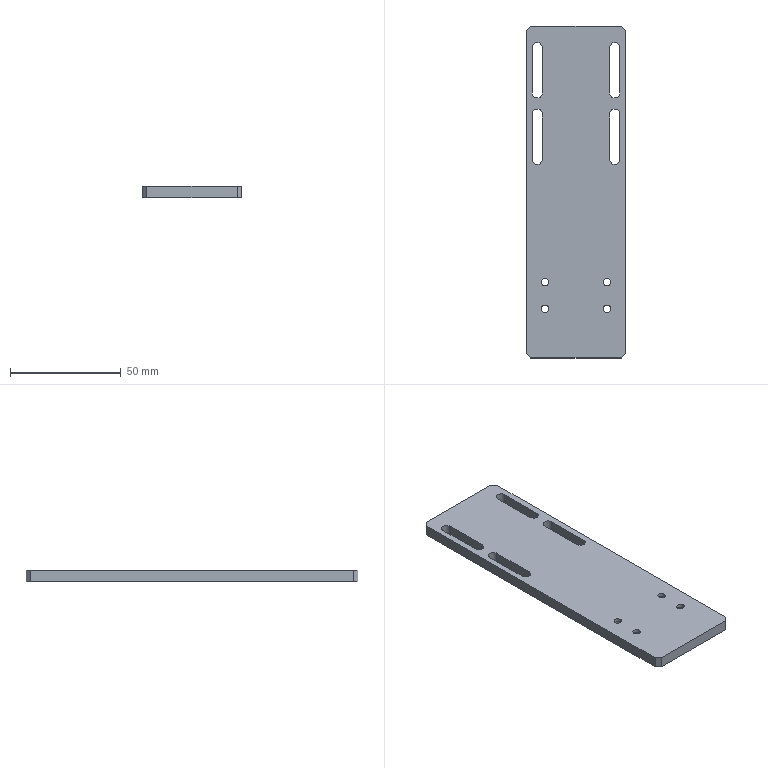Part | SolidWorks | features BaseBody 1 | 1 solid | 46 faces | box 45 x 150 x 5 mm | volume 31104 mm3 | cylinder 24 | plane 22 | commonest cylinder face diameters 3.4 x8 4.5 x8 6 x8
STEP:
#1=CARTESIAN_POINT('',(17.,-40.75,3.4));
#2=VERTEX_POINT('',#1);
#3=CARTESIAN_POINT('',(11.,-40.75,3.4));
#4=VERTEX_POINT('',#3);
#5=CARTESIAN_POINT('',(14.,-40.75,3.4));
#6=DIRECTION('',(0.,0.,-1.));
#7=DIRECTION('',(-1.,0.,0.));
#8=AXIS2_PLACEMENT_3D('',#5,#6,#7);
#9=CIRCLE('',#8,3.);
#10=EDGE_CURVE('',#2,#4,#9,.T.);
#11=ORIENTED_EDGE('',*,*,#10,.F.);
#12=CARTESIAN_POINT('',(17.,-40.75,0.));
#13=VERTEX_POINT('',#12);
#14=CARTESIAN_POINT('',(17.,-40.75,0.));
#15=DIRECTION('',(0.,0.,-1.));
#16=VECTOR('',#15,1000.);
#17=LINE('',#14,#16);
#18=EDGE_CURVE('',#2,#13,#17,.T.);
#19=ORIENTED_EDGE('',*,*,#18,.T.);
#20=CARTESIAN_POINT('',(11.,-40.75,0.));
#21=VERTEX_POINT('',#20);
#22=CARTESIAN_POINT('',(14.,-40.75,0.));
#23=DIRECTION('',(0.,0.,-1.));
#24=DIRECTION('',(-1.,0.,0.));
#25=AXIS2_PLACEMENT_3D('',#22,#23,#24);
#26=CIRCLE('',#25,3.);
#27=EDGE_CURVE('',#13,#21,#26,.T.);
#28=ORIENTED_EDGE('',*,*,#27,.T.);
#29=CARTESIAN_POINT('',(11.,-40.75,0.));
#30=DIRECTION('',(0.,0.,-1.));
#31=VECTOR('',#30,1000.);
#32=LINE('',#29,#31);
#33=EDGE_CURVE('',#4,#21,#32,.T.);
#34=ORIENTED_EDGE('',*,*,#33,.F.);
#35=EDGE_LOOP('',(#11,#19,#28,#34));
#36=FACE_OUTER_BOUND('',#35,.T.);
#37=CARTESIAN_POINT('',(14.,-40.75,0.));
#38=DIRECTION('',(0.,0.,-1.));
#39=DIRECTION('',(-1.,0.,0.));
#40=AXIS2_PLACEMENT_3D('',#37,#38,#39);
#41=CYLINDRICAL_SURFACE('',#40,3.);
#42=ADVANCED_FACE('',(#36),#41,.F.);
#43=CARTESIAN_POINT('',(15.7,-40.75,5.));
#44=VERTEX_POINT('',#43);
#45=CARTESIAN_POINT('',(12.3,-40.75,5.));
#46=VERTEX_POINT('',#45);
#47=CARTESIAN_POINT('',(14.,-40.75,5.));
#48=DIRECTION('',(0.,0.,-1.));
#49=DIRECTION('',(-1.,0.,0.));
#50=AXIS2_PLACEMENT_3D('',#47,#48,#49);
#51=CIRCLE('',#50,1.7);
#52=EDGE_CURVE('',#44,#46,#51,.T.);
#53=ORIENTED_EDGE('',*,*,#52,.F.);
#54=CARTESIAN_POINT('',(15.7,-40.75,3.4));
#55=VERTEX_POINT('',#54);
#56=CARTESIAN_POINT('',(15.7,-40.75,0.));
#57=DIRECTION('',(0.,0.,-1.));
#58=VECTOR('',#57,1000.);
#59=LINE('',#56,#58);
#60=EDGE_CURVE('',#44,#55,#59,.T.);
#61=ORIENTED_EDGE('',*,*,#60,.T.);
#62=CARTESIAN_POINT('',(12.3,-40.75,3.4));
#63=VERTEX_POINT('',#62);
#64=CARTESIAN_POINT('',(14.,-40.75,3.4));
#65=DIRECTION('',(0.,0.,-1.));
#66=DIRECTION('',(-1.,0.,0.));
#67=AXIS2_PLACEMENT_3D('',#64,#65,#66);
#68=CIRCLE('',#67,1.7);
#69=EDGE_CURVE('',#55,#63,#68,.T.);
#70=ORIENTED_EDGE('',*,*,#69,.T.);
#71=CARTESIAN_POINT('',(12.3,-40.75,0.));
#72=DIRECTION('',(0.,0.,-1.));
#73=VECTOR('',#72,1000.);
#74=LINE('',#71,#73);
#75=EDGE_CURVE('',#46,#63,#74,.T.);
#76=ORIENTED_EDGE('',*,*,#75,.F.);
#77=EDGE_LOOP('',(#53,#61,#70,#76));
#78=FACE_OUTER_BOUND('',#77,.T.);
#79=CARTESIAN_POINT('',(14.,-40.75,0.));
#80=DIRECTION('',(0.,0.,-1.));
#81=DIRECTION('',(-1.,0.,0.));
#82=AXIS2_PLACEMENT_3D('',#79,#80,#81);
#83=CYLINDRICAL_SURFACE('',#82,1.7);
#84=ADVANCED_FACE('',(#78),#83,.F.);
#85=CARTESIAN_POINT('',(-11.,-40.75,3.4));
#86=VERTEX_POINT('',#85);
#87=CARTESIAN_POINT('',(-17.,-40.75,3.4));
#88=VERTEX_POINT('',#87);
#89=CARTESIAN_POINT('',(-14.,-40.75,3.4));
#90=DIRECTION('',(0.,0.,-1.));
#91=DIRECTION('',(-1.,0.,0.));
#92=AXIS2_PLACEMENT_3D('',#89,#90,#91);
#93=CIRCLE('',#92,3.);
#94=EDGE_CURVE('',#86,#88,#93,.T.);
#95=ORIENTED_EDGE('',*,*,#94,.F.);
#96=CARTESIAN_POINT('',(-11.,-40.75,0.));
#97=VERTEX_POINT('',#96);
#98=CARTESIAN_POINT('',(-11.,-40.75,0.));
#99=DIRECTION('',(0.,0.,-1.));
#100=VECTOR('',#99,1000.);
#101=LINE('',#98,#100);
#102=EDGE_CURVE('',#86,#97,#101,.T.);
#103=ORIENTED_EDGE('',*,*,#102,.T.);
#104=CARTESIAN_POINT('',(-17.,-40.75,0.));
#105=VERTEX_POINT('',#104);
#106=CARTESIAN_POINT('',(-14.,-40.75,0.));
#107=DIRECTION('',(0.,0.,-1.));
#108=DIRECTION('',(-1.,0.,0.));
#109=AXIS2_PLACEMENT_3D('',#106,#107,#108);
#110=CIRCLE('',#109,3.);
#111=EDGE_CURVE('',#97,#105,#110,.T.);
#112=ORIENTED_EDGE('',*,*,#111,.T.);
#113=CARTESIAN_POINT('',(-17.,-40.75,0.));
#114=DIRECTION('',(0.,0.,-1.));
#115=VECTOR('',#114,1000.);
#116=LINE('',#113,#115);
#117=EDGE_CURVE('',#88,#105,#116,.T.);
#118=ORIENTED_EDGE('',*,*,#117,.F.);
#119=EDGE_LOOP('',(#95,#103,#112,#118));
#120=FACE_OUTER_BOUND('',#119,.T.);
#121=CARTESIAN_POINT('',(-14.,-40.75,0.));
#122=DIRECTION('',(0.,0.,-1.));
#123=DIRECTION('',(-1.,0.,0.));
#124=AXIS2_PLACEMENT_3D('',#121,#122,#123);
#125=CYLINDRICAL_SURFACE('',#124,3.);
#126=ADVANCED_FACE('',(#120),#125,.F.);
#127=CARTESIAN_POINT('',(-12.3,-40.75,5.));
#128=VERTEX_POINT('',#127);
#129=CARTESIAN_POINT('',(-15.7,-40.75,5.));
#130=VERTEX_POINT('',#129);
#131=CARTESIAN_POINT('',(-14.,-40.75,5.));
#132=DIRECTION('',(0.,0.,-1.));
#133=DIRECTION('',(-1.,0.,0.));
#134=AXIS2_PLACEMENT_3D('',#131,#132,#133);
#135=CIRCLE('',#134,1.7);
#136=EDGE_CURVE('',#128,#130,#135,.T.);
#137=ORIENTED_EDGE('',*,*,#136,.F.);
#138=CARTESIAN_POINT('',(-12.3,-40.75,3.4));
#139=VERTEX_POINT('',#138);
#140=CARTESIAN_POINT('',(-12.3,-40.75,0.));
#141=DIRECTION('',(0.,0.,-1.));
#142=VECTOR('',#141,1000.);
#143=LINE('',#140,#142);
#144=EDGE_CURVE('',#128,#139,#143,.T.);
#145=ORIENTED_EDGE('',*,*,#144,.T.);
#146=CARTESIAN_POINT('',(-15.7,-40.75,3.4));
#147=VERTEX_POINT('',#146);
#148=CARTESIAN_POINT('',(-14.,-40.75,3.4));
#149=DIRECTION('',(0.,0.,-1.));
#150=DIRECTION('',(-1.,0.,0.));
#151=AXIS2_PLACEMENT_3D('',#148,#149,#150);
#152=CIRCLE('',#151,1.7);
#153=EDGE_CURVE('',#139,#147,#152,.T.);
#154=ORIENTED_EDGE('',*,*,#153,.T.);
#155=CARTESIAN_POINT('',(-15.7,-40.75,0.));
#156=DIRECTION('',(0.,0.,-1.));
#157=VECTOR('',#156,1000.);
#158=LINE('',#155,#157);
#159=EDGE_CURVE('',#130,#147,#158,.T.);
#160=ORIENTED_EDGE('',*,*,#159,.F.);
#161=EDGE_LOOP('',(#137,#145,#154,#160));
#162=FACE_OUTER_BOUND('',#161,.T.);
#163=CARTESIAN_POINT('',(-14.,-40.75,0.));
#164=DIRECTION('',(0.,0.,-1.));
#165=DIRECTION('',(-1.,0.,0.));
#166=AXIS2_PLACEMENT_3D('',#163,#164,#165);
#167=CYLINDRICAL_SURFACE('',#166,1.7);
#168=ADVANCED_FACE('',(#162),#167,.F.);
#169=CARTESIAN_POINT('',(17.,-52.75,3.4));
#170=VERTEX_POINT('',#169);
#171=CARTESIAN_POINT('',(11.,-52.75,3.4));
#172=VERTEX_POINT('',#171);
#173=CARTESIAN_POINT('',(14.,-52.75,3.4));
#174=DIRECTION('',(0.,0.,-1.));
#175=DIRECTION('',(-1.,0.,0.));
#176=AXIS2_PLACEMENT_3D('',#173,#174,#175);
#177=CIRCLE('',#176,3.);
#178=EDGE_CURVE('',#170,#172,#177,.T.);
#179=ORIENTED_EDGE('',*,*,#178,.F.);
#180=CARTESIAN_POINT('',(17.,-52.75,0.));
#181=VERTEX_POINT('',#180);
#182=CARTESIAN_POINT('',(17.,-52.75,0.));
#183=DIRECTION('',(0.,0.,-1.));
#184=VECTOR('',#183,1000.);
#185=LINE('',#182,#184);
#186=EDGE_CURVE('',#170,#181,#185,.T.);
#187=ORIENTED_EDGE('',*,*,#186,.T.);
#188=CARTESIAN_POINT('',(11.,-52.75,0.));
#189=VERTEX_POINT('',#188);
#190=CARTESIAN_POINT('',(14.,-52.75,0.));
#191=DIRECTION('',(0.,0.,-1.));
#192=DIRECTION('',(-1.,0.,0.));
#193=AXIS2_PLACEMENT_3D('',#190,#191,#192);
#194=CIRCLE('',#193,3.);
#195=EDGE_CURVE('',#181,#189,#194,.T.);
#196=ORIENTED_EDGE('',*,*,#195,.T.);
#197=CARTESIAN_POINT('',(11.,-52.75,0.));
#198=DIRECTION('',(0.,0.,-1.));
#199=VECTOR('',#198,1000.);
#200=LINE('',#197,#199);
#201=EDGE_CURVE('',#172,#189,#200,.T.);
#202=ORIENTED_EDGE('',*,*,#201,.F.);
#203=EDGE_LOOP('',(#179,#187,#196,#202));
#204=FACE_OUTER_BOUND('',#203,.T.);
#205=CARTESIAN_POINT('',(14.,-52.75,0.));
#206=DIRECTION('',(0.,0.,-1.));
#207=DIRECTION('',(-1.,0.,0.));
#208=AXIS2_PLACEMENT_3D('',#205,#206,#207);
#209=CYLINDRICAL_SURFACE('',#208,3.);
#210=ADVANCED_FACE('',(#204),#209,.F.);
#211=CARTESIAN_POINT('',(15.7,-52.75,5.));
#212=VERTEX_POINT('',#211);
#213=CARTESIAN_POINT('',(12.3,-52.75,5.));
#214=VERTEX_POINT('',#213);
#215=CARTESIAN_POINT('',(14.,-52.75,5.));
#216=DIRECTION('',(0.,0.,-1.));
#217=DIRECTION('',(-1.,0.,0.));
#218=AXIS2_PLACEMENT_3D('',#215,#216,#217);
#219=CIRCLE('',#218,1.7);
#220=EDGE_CURVE('',#212,#214,#219,.T.);
#221=ORIENTED_EDGE('',*,*,#220,.F.);
#222=CARTESIAN_POINT('',(15.7,-52.75,3.4));
#223=VERTEX_POINT('',#222);
#224=CARTESIAN_POINT('',(15.7,-52.75,0.));
#225=DIRECTION('',(0.,0.,-1.));
#226=VECTOR('',#225,1000.);
#227=LINE('',#224,#226);
#228=EDGE_CURVE('',#212,#223,#227,.T.);
#229=ORIENTED_EDGE('',*,*,#228,.T.);
#230=CARTESIAN_POINT('',(12.3,-52.75,3.4));
#231=VERTEX_POINT('',#230);
#232=CARTESIAN_POINT('',(14.,-52.75,3.4));
#233=DIRECTION('',(0.,0.,-1.));
#234=DIRECTION('',(-1.,0.,0.));
#235=AXIS2_PLACEMENT_3D('',#232,#233,#234);
#236=CIRCLE('',#235,1.7);
#237=EDGE_CURVE('',#223,#231,#236,.T.);
#238=ORIENTED_EDGE('',*,*,#237,.T.);
#239=CARTESIAN_POINT('',(12.3,-52.75,0.));
#240=DIRECTION('',(0.,0.,-1.));
#241=VECTOR('',#240,1000.);
#242=LINE('',#239,#241);
#243=EDGE_CURVE('',#214,#231,#242,.T.);
#244=ORIENTED_EDGE('',*,*,#243,.F.);
#245=EDGE_LOOP('',(#221,#229,#238,#244));
#246=FACE_OUTER_BOUND('',#245,.T.);
#247=CARTESIAN_POINT('',(14.,-52.75,0.));
#248=DIRECTION('',(0.,0.,-1.));
#249=DIRECTION('',(-1.,0.,0.));
#250=AXIS2_PLACEMENT_3D('',#247,#248,#249);
#251=CYLINDRICAL_SURFACE('',#250,1.7);
#252=ADVANCED_FACE('',(#246),#251,.F.);
#253=CARTESIAN_POINT('',(-11.,-52.75,3.4));
#254=VERTEX_POINT('',#253);
#255=CARTESIAN_POINT('',(-17.,-52.75,3.4));
#256=VERTEX_POINT('',#255);
#257=CARTESIAN_POINT('',(-14.,-52.75,3.4));
#258=DIRECTION('',(0.,0.,-1.));
#259=DIRECTION('',(-1.,0.,0.));
#260=AXIS2_PLACEMENT_3D('',#257,#258,#259);
#261=CIRCLE('',#260,3.);
#262=EDGE_CURVE('',#254,#256,#261,.T.);
#263=ORIENTED_EDGE('',*,*,#262,.F.);
#264=CARTESIAN_POINT('',(-11.,-52.75,0.));
#265=VERTEX_POINT('',#264);
#266=CARTESIAN_POINT('',(-11.,-52.75,0.));
#267=DIRECTION('',(0.,0.,-1.));
#268=VECTOR('',#267,1000.);
#269=LINE('',#266,#268);
#270=EDGE_CURVE('',#254,#265,#269,.T.);
#271=ORIENTED_EDGE('',*,*,#270,.T.);
#272=CARTESIAN_POINT('',(-17.,-52.75,0.));
#273=VERTEX_POINT('',#272);
#274=CARTESIAN_POINT('',(-14.,-52.75,0.));
#275=DIRECTION('',(0.,0.,-1.));
#276=DIRECTION('',(-1.,0.,0.));
#277=AXIS2_PLACEMENT_3D('',#274,#275,#276);
#278=CIRCLE('',#277,3.);
#279=EDGE_CURVE('',#265,#273,#278,.T.);
#280=ORIENTED_EDGE('',*,*,#279,.T.);
#281=CARTESIAN_POINT('',(-17.,-52.75,0.));
#282=DIRECTION('',(0.,0.,-1.));
#283=VECTOR('',#282,1000.);
#284=LINE('',#281,#283);
#285=EDGE_CURVE('',#256,#273,#284,.T.);
#286=ORIENTED_EDGE('',*,*,#285,.F.);
#287=EDGE_LOOP('',(#263,#271,#280,#286));
#288=FACE_OUTER_BOUND('',#287,.T.);
#289=CARTESIAN_POINT('',(-14.,-52.75,0.));
#290=DIRECTION('',(0.,0.,-1.));
#291=DIRECTION('',(-1.,0.,0.));
#292=AXIS2_PLACEMENT_3D('',#289,#290,#291);
#293=CYLINDRICAL_SURFACE('',#292,3.);
#294=ADVANCED_FACE('',(#288),#293,.F.);
#295=CARTESIAN_POINT('',(-12.3,-52.75,5.));
#296=VERTEX_POINT('',#295);
#297=CARTESIAN_POINT('',(-15.7,-52.75,5.));
#298=VERTEX_POINT('',#297);
#299=CARTESIAN_POINT('',(-14.,-52.75,5.));
#300=DIRECTION('',(0.,0.,-1.));
#301=DIRECTION('',(-1.,0.,0.));
#302=AXIS2_PLACEMENT_3D('',#299,#300,#301);
#303=CIRCLE('',#302,1.7);
#304=EDGE_CURVE('',#296,#298,#303,.T.);
#305=ORIENTED_EDGE('',*,*,#304,.F.);
#306=CARTESIAN_POINT('',(-12.3,-52.75,3.4));
#307=VERTEX_POINT('',#306);
#308=CARTESIAN_POINT('',(-12.3,-52.75,0.));
#309=DIRECTION('',(0.,0.,-1.));
#310=VECTOR('',#309,1000.);
#311=LINE('',#308,#310);
#312=EDGE_CURVE('',#296,#307,#311,.T.);
#313=ORIENTED_EDGE('',*,*,#312,.T.);
#314=CARTESIAN_POINT('',(-15.7,-52.75,3.4));
#315=VERTEX_POINT('',#314);
#316=CARTESIAN_POINT('',(-14.,-52.75,3.4));
#317=DIRECTION('',(0.,0.,-1.));
#318=DIRECTION('',(-1.,0.,0.));
#319=AXIS2_PLACEMENT_3D('',#316,#317,#318);
#320=CIRCLE('',#319,1.7);
#321=EDGE_CURVE('',#307,#315,#320,.T.);
#322=ORIENTED_EDGE('',*,*,#321,.T.);
#323=CARTESIAN_POINT('',(-15.7,-52.75,0.));
#324=DIRECTION('',(0.,0.,-1.));
#325=VECTOR('',#324,1000.);
#326=LINE('',#323,#325);
#327=EDGE_CURVE('',#298,#315,#326,.T.);
#328=ORIENTED_EDGE('',*,*,#327,.F.);
#329=EDGE_LOOP('',(#305,#313,#322,#328));
#330=FACE_OUTER_BOUND('',#329,.T.);
#331=CARTESIAN_POINT('',(-14.,-52.75,0.));
#332=DIRECTION('',(0.,0.,-1.));
#333=DIRECTION('',(-1.,0.,0.));
#334=AXIS2_PLACEMENT_3D('',#331,#332,#333);
#335=CYLINDRICAL_SURFACE('',#334,1.7);
#336=ADVANCED_FACE('',(#330),#335,.F.);
#337=CARTESIAN_POINT('',(14.,-40.75,3.4));
#338=DIRECTION('',(0.,0.,-1.));
#339=DIRECTION('',(-1.,0.,0.));
#340=AXIS2_PLACEMENT_3D('',#337,#338,#339);
#341=CIRCLE('',#340,1.7);
#342=EDGE_CURVE('',#63,#55,#341,.T.);
#343=ORIENTED_EDGE('',*,*,#342,.F.);
#344=ORIENTED_EDGE('',*,*,#69,.F.);
#345=EDGE_LOOP('',(#343,#344));
#346=FACE_BOUND('',#345,.T.);
#347=CARTESIAN_POINT('',(14.,-40.75,3.4));
#348=DIRECTION('',(0.,0.,-1.));
#349=DIRECTION('',(-1.,0.,0.));
#350=AXIS2_PLACEMENT_3D('',#347,#348,#349);
#351=CIRCLE('',#350,3.);
#352=EDGE_CURVE('',#4,#2,#351,.T.);
#353=ORIENTED_EDGE('',*,*,#352,.T.);
#354=ORIENTED_EDGE('',*,*,#10,.T.);
#355=EDGE_LOOP('',(#353,#354));
#356=FACE_OUTER_BOUND('',#355,.T.);
#357=CARTESIAN_POINT('',(15.7,-40.75,3.4));
#358=DIRECTION('',(0.,0.,1.));
#359=DIRECTION('',(1.,0.,0.));
#360=AXIS2_PLACEMENT_3D('',#357,#358,#359);
#361=PLANE('',#360);
#362=ADVANCED_FACE('',(#346,#356),#361,.F.);
#363=CARTESIAN_POINT('',(-14.,-40.75,3.4));
#364=DIRECTION('',(0.,0.,-1.));
#365=DIRECTION('',(-1.,0.,0.));
#366=AXIS2_PLACEMENT_3D('',#363,#364,#365);
#367=CIRCLE('',#366,1.7);
#368=EDGE_CURVE('',#147,#139,#367,.T.);
#369=ORIENTED_EDGE('',*,*,#368,.F.);
#370=ORIENTED_EDGE('',*,*,#153,.F.);
#371=EDGE_LOOP('',(#369,#370));
#372=FACE_BOUND('',#371,.T.);
#373=CARTESIAN_POINT('',(-14.,-40.75,3.4));
#374=DIRECTION('',(0.,0.,-1.));
#375=DIRECTION('',(-1.,0.,0.));
#376=AXIS2_PLACEMENT_3D('',#373,#374,#375);
#377=CIRCLE('',#376,3.);
#378=EDGE_CURVE('',#88,#86,#377,.T.);
#379=ORIENTED_EDGE('',*,*,#378,.T.);
#380=ORIENTED_EDGE('',*,*,#94,.T.);
#381=EDGE_LOOP('',(#379,#380));
#382=FACE_OUTER_BOUND('',#381,.T.);
#383=CARTESIAN_POINT('',(-12.3,-40.75,3.4));
#384=DIRECTION('',(0.,0.,1.));
#385=DIRECTION('',(1.,0.,0.));
#386=AXIS2_PLACEMENT_3D('',#383,#384,#385);
#387=PLANE('',#386);
#388=ADVANCED_FACE('',(#372,#382),#387,.F.);
#389=CARTESIAN_POINT('',(14.,-52.75,3.4));
#390=DIRECTION('',(0.,0.,-1.));
#391=DIRECTION('',(-1.,0.,0.));
#392=AXIS2_PLACEMENT_3D('',#389,#390,#391);
#393=CIRCLE('',#392,1.7);
#394=EDGE_CURVE('',#231,#223,#393,.T.);
#395=ORIENTED_EDGE('',*,*,#394,.F.);
#396=ORIENTED_EDGE('',*,*,#237,.F.);
#397=EDGE_LOOP('',(#395,#396));
#398=FACE_BOUND('',#397,.T.);
#399=CARTESIAN_POINT('',(14.,-52.75,3.4));
#400=DIRECTION('',(0.,0.,-1.));
#401=DIRECTION('',(-1.,0.,0.));
#402=AXIS2_PLACEMENT_3D('',#399,#400,#401);
#403=CIRCLE('',#402,3.);
#404=EDGE_CURVE('',#172,#170,#403,.T.);
#405=ORIENTED_EDGE('',*,*,#404,.T.);
#406=ORIENTED_EDGE('',*,*,#178,.T.);
#407=EDGE_LOOP('',(#405,#406));
#408=FACE_OUTER_BOUND('',#407,.T.);
#409=CARTESIAN_POINT('',(15.7,-52.75,3.4));
#410=DIRECTION('',(0.,0.,1.));
#411=DIRECTION('',(1.,0.,0.));
#412=AXIS2_PLACEMENT_3D('',#409,#410,#411);
#413=PLANE('',#412);
#414=ADVANCED_FACE('',(#398,#408),#413,.F.);
#415=CARTESIAN_POINT('',(-14.,-52.75,3.4));
#416=DIRECTION('',(0.,0.,-1.));
#417=DIRECTION('',(-1.,0.,0.));
#418=AXIS2_PLACEMENT_3D('',#415,#416,#417);
#419=CIRCLE('',#418,1.7);
#420=EDGE_CURVE('',#315,#307,#419,.T.);
#421=ORIENTED_EDGE('',*,*,#420,.F.);
#422=ORIENTED_EDGE('',*,*,#321,.F.);
#423=EDGE_LOOP('',(#421,#422));
#424=FACE_BOUND('',#423,.T.);
#425=CARTESIAN_POINT('',(-14.,-52.75,3.4));
#426=DIRECTION('',(0.,0.,-1.));
#427=DIRECTION('',(-1.,0.,0.));
#428=AXIS2_PLACEMENT_3D('',#425,#426,#427);
#429=CIRCLE('',#428,3.);
#430=EDGE_CURVE('',#256,#254,#429,.T.);
#431=ORIENTED_EDGE('',*,*,#430,.T.);
#432=ORIENTED_EDGE('',*,*,#262,.T.);
#433=EDGE_LOOP('',(#431,#432));
#434=FACE_OUTER_BOUND('',#433,.T.);
#435=CARTESIAN_POINT('',(-12.3,-52.75,3.4));
#436=DIRECTION('',(0.,0.,1.));
#437=DIRECTION('',(1.,0.,0.));
#438=AXIS2_PLACEMENT_3D('',#435,#436,#437);
#439=PLANE('',#438);
#440=ADVANCED_FACE('',(#424,#434),#439,.F.);
#441=CARTESIAN_POINT('',(15.25,65.25,0.));
#442=VERTEX_POINT('',#441);
#443=CARTESIAN_POINT('',(15.25,65.25,5.));
#444=VERTEX_POINT('',#443);
#445=CARTESIAN_POINT('',(15.25,65.25,0.));
#446=DIRECTION('',(0.,0.,1.));
#447=VECTOR('',#446,1000.);
#448=LINE('',#445,#447);
#449=EDGE_CURVE('',#442,#444,#448,.T.);
#450=ORIENTED_EDGE('',*,*,#449,.T.);
#451=CARTESIAN_POINT('',(15.25,44.75,5.));
#452=VERTEX_POINT('',#451);
#453=CARTESIAN_POINT('',(15.25,44.75,5.));
#454=DIRECTION('',(0.,1.,0.));
#455=VECTOR('',#454,1000.);
#456=LINE('',#453,#455);
#457=EDGE_CURVE('',#452,#444,#456,.T.);
#458=ORIENTED_EDGE('',*,*,#457,.F.);
#459=CARTESIAN_POINT('',(15.25,44.75,0.));
#460=VERTEX_POINT('',#459);
#461=CARTESIAN_POINT('',(15.25,44.75,0.));
#462=DIRECTION('',(0.,0.,-1.));
#463=VECTOR('',#462,1000.);
#464=LINE('',#461,#463);
#465=EDGE_CURVE('',#452,#460,#464,.T.);
#466=ORIENTED_EDGE('',*,*,#465,.T.);
#467=CARTESIAN_POINT('',(15.25,44.75,0.));
#468=DIRECTION('',(0.,1.,0.));
#469=VECTOR('',#468,1000.);
#470=LINE('',#467,#469);
#471=EDGE_CURVE('',#460,#442,#470,.T.);
#472=ORIENTED_EDGE('',*,*,#471,.T.);
#473=EDGE_LOOP('',(#450,#458,#466,#472));
#474=FACE_OUTER_BOUND('',#473,.T.);
#475=CARTESIAN_POINT('',(15.25,44.75,0.));
#476=DIRECTION('',(-1.,0.,0.));
#477=DIRECTION('',(0.,1.,0.));
#478=AXIS2_PLACEMENT_3D('',#475,#476,#477);
#479=PLANE('',#478);
#480=ADVANCED_FACE('',(#474),#479,.F.);
#481=CARTESIAN_POINT('',(19.75,65.25,0.));
#482=VERTEX_POINT('',#481);
#483=CARTESIAN_POINT('',(19.75,65.25,5.));
#484=VERTEX_POINT('',#483);
#485=CARTESIAN_POINT('',(19.75,65.25,5.));
#486=DIRECTION('',(0.,0.,1.));
#487=VECTOR('',#486,1000.);
#488=LINE('',#485,#487);
#489=EDGE_CURVE('',#482,#484,#488,.T.);
#490=ORIENTED_EDGE('',*,*,#489,.F.);
#491=CARTESIAN_POINT('',(19.75,44.75,0.));
#492=VERTEX_POINT('',#491);
#493=CARTESIAN_POINT('',(19.75,44.75,0.));
#494=DIRECTION('',(0.,1.,0.));
#495=VECTOR('',#494,1000.);
#496=LINE('',#493,#495);
#497=EDGE_CURVE('',#492,#482,#496,.T.);
#498=ORIENTED_EDGE('',*,*,#497,.F.);
#499=CARTESIAN_POINT('',(19.75,44.75,5.));
#500=VERTEX_POINT('',#499);
#501=CARTESIAN_POINT('',(19.75,44.75,5.));
#502=DIRECTION('',(0.,0.,1.));
#503=VECTOR('',#502,1000.);
#504=LINE('',#501,#503);
#505=EDGE_CURVE('',#492,#500,#504,.T.);
#506=ORIENTED_EDGE('',*,*,#505,.T.);
#507=CARTESIAN_POINT('',(19.75,44.75,5.));
#508=DIRECTION('',(0.,1.,0.));
#509=VECTOR('',#508,1000.);
#510=LINE('',#507,#509);
#511=EDGE_CURVE('',#500,#484,#510,.T.);
#512=ORIENTED_EDGE('',*,*,#511,.T.);
#513=EDGE_LOOP('',(#490,#498,#506,#512));
#514=FACE_OUTER_BOUND('',#513,.T.);
#515=CARTESIAN_POINT('',(19.75,44.75,5.));
#516=DIRECTION('',(-1.,0.,0.));
#517=DIRECTION('',(0.,0.,1.));
#518=AXIS2_PLACEMENT_3D('',#515,#516,#517);
#519=PLANE('',#518);
#520=ADVANCED_FACE('',(#514),#519,.T.);
#521=CARTESIAN_POINT('',(17.5,44.75,5.));
#522=DIRECTION('',(0.,0.,-1.));
#523=DIRECTION('',(-1.,0.,0.));
#524=AXIS2_PLACEMENT_3D('',#521,#522,#523);
#525=CIRCLE('',#524,2.25);
#526=EDGE_CURVE('',#500,#452,#525,.T.);
#527=ORIENTED_EDGE('',*,*,#526,.F.);
#528=ORIENTED_EDGE('',*,*,#505,.F.);
#529=CARTESIAN_POINT('',(17.5,44.75,0.));
#530=DIRECTION('',(0.,0.,-1.));
#531=DIRECTION('',(-1.,0.,0.));
#532=AXIS2_PLACEMENT_3D('',#529,#530,#531);
#533=CIRCLE('',#532,2.25);
#534=EDGE_CURVE('',#492,#460,#533,.T.);
#535=ORIENTED_EDGE('',*,*,#534,.T.);
#536=ORIENTED_EDGE('',*,*,#465,.F.);
#537=EDGE_LOOP('',(#527,#528,#535,#536));
#538=FACE_OUTER_BOUND('',#537,.T.);
#539=CARTESIAN_POINT('',(17.5,44.75,0.));
#540=DIRECTION('',(0.,0.,-1.));
#541=DIRECTION('',(-1.,0.,0.));
#542=AXIS2_PLACEMENT_3D('',#539,#540,#541);
#543=CYLINDRICAL_SURFACE('',#542,2.25);
#544=ADVANCED_FACE('',(#538),#543,.F.);
#545=CARTESIAN_POINT('',(17.5,65.25,0.));
#546=DIRECTION('',(0.,0.,-1.));
#547=DIRECTION('',(-1.,0.,0.));
#548=AXIS2_PLACEMENT_3D('',#545,#546,#547);
#549=CIRCLE('',#548,2.25);
#550=EDGE_CURVE('',#442,#482,#549,.T.);
#551=ORIENTED_EDGE('',*,*,#550,.T.);
#552=ORIENTED_EDGE('',*,*,#489,.T.);
#553=CARTESIAN_POINT('',(17.5,65.25,5.));
#554=DIRECTION('',(0.,0.,-1.));
#555=DIRECTION('',(-1.,0.,0.));
#556=AXIS2_PLACEMENT_3D('',#553,#554,#555);
#557=CIRCLE('',#556,2.25);
#558=EDGE_CURVE('',#444,#484,#557,.T.);
#559=ORIENTED_EDGE('',*,*,#558,.F.);
#560=ORIENTED_EDGE('',*,*,#449,.F.);
#561=EDGE_LOOP('',(#551,#552,#559,#560));
#562=FACE_OUTER_BOUND('',#561,.T.);
#563=CARTESIAN_POINT('',(17.5,65.25,0.));
#564=DIRECTION('',(0.,0.,-1.));
#565=DIRECTION('',(-1.,0.,0.));
#566=AXIS2_PLACEMENT_3D('',#563,#564,#565);
#567=CYLINDRICAL_SURFACE('',#566,2.25);
#568=ADVANCED_FACE('',(#562),#567,.F.);
#569=CARTESIAN_POINT('',(15.25,35.25,0.));
#570=VERTEX_POINT('',#569);
#571=CARTESIAN_POINT('',(15.25,35.25,5.));
#572=VERTEX_POINT('',#571);
#573=CARTESIAN_POINT('',(15.25,35.25,0.));
#574=DIRECTION('',(0.,0.,1.));
#575=VECTOR('',#574,1000.);
#576=LINE('',#573,#575);
#577=EDGE_CURVE('',#570,#572,#576,.T.);
#578=ORIENTED_EDGE('',*,*,#577,.T.);
#579=CARTESIAN_POINT('',(15.25,14.75,5.));
#580=VERTEX_POINT('',#579);
#581=CARTESIAN_POINT('',(15.25,14.75,5.));
#582=DIRECTION('',(0.,1.,0.));
#583=VECTOR('',#582,1000.);
#584=LINE('',#581,#583);
#585=EDGE_CURVE('',#580,#572,#584,.T.);
#586=ORIENTED_EDGE('',*,*,#585,.F.);
#587=CARTESIAN_POINT('',(15.25,14.75,0.));
#588=VERTEX_POINT('',#587);
#589=CARTESIAN_POINT('',(15.25,14.75,0.));
#590=DIRECTION('',(0.,0.,-1.));
#591=VECTOR('',#590,1000.);
#592=LINE('',#589,#591);
#593=EDGE_CURVE('',#580,#588,#592,.T.);
#594=ORIENTED_EDGE('',*,*,#593,.T.);
#595=CARTESIAN_POINT('',(15.25,14.75,0.));
#596=DIRECTION('',(0.,1.,0.));
#597=VECTOR('',#596,1000.);
#598=LINE('',#595,#597);
#599=EDGE_CURVE('',#588,#570,#598,.T.);
#600=ORIENTED_EDGE('',*,*,#599,.T.);
#601=EDGE_LOOP('',(#578,#586,#594,#600));
#602=FACE_OUTER_BOUND('',#601,.T.);
#603=CARTESIAN_POINT('',(15.25,14.75,0.));
#604=DIRECTION('',(-1.,0.,0.));
#605=DIRECTION('',(0.,1.,0.));
#606=AXIS2_PLACEMENT_3D('',#603,#604,#605);
#607=PLANE('',#606);
#608=ADVANCED_FACE('',(#602),#607,.F.);
#609=CARTESIAN_POINT('',(19.75,35.25,0.));
#610=VERTEX_POINT('',#609);
#611=CARTESIAN_POINT('',(19.75,35.25,5.));
#612=VERTEX_POINT('',#611);
#613=CARTESIAN_POINT('',(19.75,35.25,5.));
#614=DIRECTION('',(0.,0.,1.));
#615=VECTOR('',#614,1000.);
#616=LINE('',#613,#615);
#617=EDGE_CURVE('',#610,#612,#616,.T.);
#618=ORIENTED_EDGE('',*,*,#617,.F.);
#619=CARTESIAN_POINT('',(19.75,14.75,0.));
#620=VERTEX_POINT('',#619);
#621=CARTESIAN_POINT('',(19.75,14.75,0.));
#622=DIRECTION('',(0.,1.,0.));
#623=VECTOR('',#622,1000.);
#624=LINE('',#621,#623);
#625=EDGE_CURVE('',#620,#610,#624,.T.);
#626=ORIENTED_EDGE('',*,*,#625,.F.);
#627=CARTESIAN_POINT('',(19.75,14.75,5.));
#628=VERTEX_POINT('',#627);
#629=CARTESIAN_POINT('',(19.75,14.75,5.));
#630=DIRECTION('',(0.,0.,1.));
#631=VECTOR('',#630,1000.);
#632=LINE('',#629,#631);
#633=EDGE_CURVE('',#620,#628,#632,.T.);
#634=ORIENTED_EDGE('',*,*,#633,.T.);
#635=CARTESIAN_POINT('',(19.75,14.75,5.));
#636=DIRECTION('',(0.,1.,0.));
#637=VECTOR('',#636,1000.);
#638=LINE('',#635,#637);
#639=EDGE_CURVE('',#628,#612,#638,.T.);
#640=ORIENTED_EDGE('',*,*,#639,.T.);
#641=EDGE_LOOP('',(#618,#626,#634,#640));
#642=FACE_OUTER_BOUND('',#641,.T.);
#643=CARTESIAN_POINT('',(19.75,14.75,5.));
#644=DIRECTION('',(-1.,0.,0.));
#645=DIRECTION('',(0.,0.,1.));
#646=AXIS2_PLACEMENT_3D('',#643,#644,#645);
#647=PLANE('',#646);
#648=ADVANCED_FACE('',(#642),#647,.T.);
#649=CARTESIAN_POINT('',(17.5,14.75,5.));
#650=DIRECTION('',(0.,0.,-1.));
#651=DIRECTION('',(-1.,0.,0.));
#652=AXIS2_PLACEMENT_3D('',#649,#650,#651);
#653=CIRCLE('',#652,2.25);
#654=EDGE_CURVE('',#628,#580,#653,.T.);
#655=ORIENTED_EDGE('',*,*,#654,.F.);
#656=ORIENTED_EDGE('',*,*,#633,.F.);
#657=CARTESIAN_POINT('',(17.5,14.75,0.));
#658=DIRECTION('',(0.,0.,-1.));
#659=DIRECTION('',(-1.,0.,0.));
#660=AXIS2_PLACEMENT_3D('',#657,#658,#659);
#661=CIRCLE('',#660,2.25);
#662=EDGE_CURVE('',#620,#588,#661,.T.);
#663=ORIENTED_EDGE('',*,*,#662,.T.);
#664=ORIENTED_EDGE('',*,*,#593,.F.);
#665=EDGE_LOOP('',(#655,#656,#663,#664));
#666=FACE_OUTER_BOUND('',#665,.T.);
#667=CARTESIAN_POINT('',(17.5,14.75,0.));
#668=DIRECTION('',(0.,0.,-1.));
#669=DIRECTION('',(-1.,0.,0.));
#670=AXIS2_PLACEMENT_3D('',#667,#668,#669);
#671=CYLINDRICAL_SURFACE('',#670,2.25);
#672=ADVANCED_FACE('',(#666),#671,.F.);
#673=CARTESIAN_POINT('',(17.5,35.25,0.));
#674=DIRECTION('',(0.,0.,-1.));
#675=DIRECTION('',(-1.,0.,0.));
#676=AXIS2_PLACEMENT_3D('',#673,#674,#675);
#677=CIRCLE('',#676,2.25);
#678=EDGE_CURVE('',#570,#610,#677,.T.);
#679=ORIENTED_EDGE('',*,*,#678,.T.);
#680=ORIENTED_EDGE('',*,*,#617,.T.);
#681=CARTESIAN_POINT('',(17.5,35.25,5.));
#682=DIRECTION('',(0.,0.,-1.));
#683=DIRECTION('',(-1.,0.,0.));
#684=AXIS2_PLACEMENT_3D('',#681,#682,#683);
#685=CIRCLE('',#684,2.25);
#686=EDGE_CURVE('',#572,#612,#685,.T.);
#687=ORIENTED_EDGE('',*,*,#686,.F.);
#688=ORIENTED_EDGE('',*,*,#577,.F.);
#689=EDGE_LOOP('',(#679,#680,#687,#688));
#690=FACE_OUTER_BOUND('',#689,.T.);
#691=CARTESIAN_POINT('',(17.5,35.25,0.));
#692=DIRECTION('',(0.,0.,-1.));
#693=DIRECTION('',(-1.,0.,0.));
#694=AXIS2_PLACEMENT_3D('',#691,#692,#693);
#695=CYLINDRICAL_SURFACE('',#694,2.25);
#696=ADVANCED_FACE('',(#690),#695,.F.);
#697=CARTESIAN_POINT('',(-19.75,35.25,0.));
#698=VERTEX_POINT('',#697);
#699=CARTESIAN_POINT('',(-19.75,35.25,5.));
#700=VERTEX_POINT('',#699);
#701=CARTESIAN_POINT('',(-19.75,35.25,0.));
#702=DIRECTION('',(0.,0.,1.));
#703=VECTOR('',#702,1000.);
#704=LINE('',#701,#703);
#705=EDGE_CURVE('',#698,#700,#704,.T.);
#706=ORIENTED_EDGE('',*,*,#705,.T.);
#707=CARTESIAN_POINT('',(-19.75,14.75,5.));
#708=VERTEX_POINT('',#707);
#709=CARTESIAN_POINT('',(-19.75,14.75,5.));
#710=DIRECTION('',(0.,1.,0.));
#711=VECTOR('',#710,1000.);
#712=LINE('',#709,#711);
#713=EDGE_CURVE('',#708,#700,#712,.T.);
#714=ORIENTED_EDGE('',*,*,#713,.F.);
#715=CARTESIAN_POINT('',(-19.75,14.75,0.));
#716=VERTEX_POINT('',#715);
#717=CARTESIAN_POINT('',(-19.75,14.75,0.));
#718=DIRECTION('',(0.,0.,-1.));
#719=VECTOR('',#718,1000.);
#720=LINE('',#717,#719);
#721=EDGE_CURVE('',#708,#716,#720,.T.);
#722=ORIENTED_EDGE('',*,*,#721,.T.);
#723=CARTESIAN_POINT('',(-19.75,14.75,0.));
#724=DIRECTION('',(0.,1.,0.));
#725=VECTOR('',#724,1000.);
#726=LINE('',#723,#725);
#727=EDGE_CURVE('',#716,#698,#726,.T.);
#728=ORIENTED_EDGE('',*,*,#727,.T.);
#729=EDGE_LOOP('',(#706,#714,#722,#728));
#730=FACE_OUTER_BOUND('',#729,.T.);
#731=CARTESIAN_POINT('',(-19.75,14.75,0.));
#732=DIRECTION('',(-1.,0.,0.));
#733=DIRECTION('',(0.,1.,0.));
#734=AXIS2_PLACEMENT_3D('',#731,#732,#733);
#735=PLANE('',#734);
#736=ADVANCED_FACE('',(#730),#735,.F.);
#737=CARTESIAN_POINT('',(-15.25,35.25,0.));
#738=VERTEX_POINT('',#737);
#739=CARTESIAN_POINT('',(-15.25,35.25,5.));
#740=VERTEX_POINT('',#739);
#741=CARTESIAN_POINT('',(-15.25,35.25,5.));
#742=DIRECTION('',(0.,0.,1.));
#743=VECTOR('',#742,1000.);
#744=LINE('',#741,#743);
#745=EDGE_CURVE('',#738,#740,#744,.T.);
#746=ORIENTED_EDGE('',*,*,#745,.F.);
#747=CARTESIAN_POINT('',(-15.25,14.75,0.));
#748=VERTEX_POINT('',#747);
#749=CARTESIAN_POINT('',(-15.25,14.75,0.));
#750=DIRECTION('',(0.,1.,0.));
#751=VECTOR('',#750,1000.);
#752=LINE('',#749,#751);
#753=EDGE_CURVE('',#748,#738,#752,.T.);
#754=ORIENTED_EDGE('',*,*,#753,.F.);
#755=CARTESIAN_POINT('',(-15.25,14.75,5.));
#756=VERTEX_POINT('',#755);
#757=CARTESIAN_POINT('',(-15.25,14.75,5.));
#758=DIRECTION('',(0.,0.,1.));
#759=VECTOR('',#758,1000.);
#760=LINE('',#757,#759);
#761=EDGE_CURVE('',#748,#756,#760,.T.);
#762=ORIENTED_EDGE('',*,*,#761,.T.);
#763=CARTESIAN_POINT('',(-15.25,14.75,5.));
#764=DIRECTION('',(0.,1.,0.));
#765=VECTOR('',#764,1000.);
#766=LINE('',#763,#765);
#767=EDGE_CURVE('',#756,#740,#766,.T.);
#768=ORIENTED_EDGE('',*,*,#767,.T.);
#769=EDGE_LOOP('',(#746,#754,#762,#768));
#770=FACE_OUTER_BOUND('',#769,.T.);
#771=CARTESIAN_POINT('',(-15.25,14.75,5.));
#772=DIRECTION('',(-1.,0.,0.));
#773=DIRECTION('',(0.,0.,1.));
#774=AXIS2_PLACEMENT_3D('',#771,#772,#773);
#775=PLANE('',#774);
#776=ADVANCED_FACE('',(#770),#775,.T.);
#777=CARTESIAN_POINT('',(-17.5,14.75,5.));
#778=DIRECTION('',(0.,0.,-1.));
#779=DIRECTION('',(-1.,0.,0.));
#780=AXIS2_PLACEMENT_3D('',#777,#778,#779);
#781=CIRCLE('',#780,2.25);
#782=EDGE_CURVE('',#756,#708,#781,.T.);
#783=ORIENTED_EDGE('',*,*,#782,.F.);
#784=ORIENTED_EDGE('',*,*,#761,.F.);
#785=CARTESIAN_POINT('',(-17.5,14.75,0.));
#786=DIRECTION('',(0.,0.,-1.));
#787=DIRECTION('',(-1.,0.,0.));
#788=AXIS2_PLACEMENT_3D('',#785,#786,#787);
#789=CIRCLE('',#788,2.25);
#790=EDGE_CURVE('',#748,#716,#789,.T.);
#791=ORIENTED_EDGE('',*,*,#790,.T.);
#792=ORIENTED_EDGE('',*,*,#721,.F.);
#793=EDGE_LOOP('',(#783,#784,#791,#792));
#794=FACE_OUTER_BOUND('',#793,.T.);
#795=CARTESIAN_POINT('',(-17.5,14.75,0.));
#796=DIRECTION('',(0.,0.,-1.));
#797=DIRECTION('',(-1.,0.,0.));
#798=AXIS2_PLACEMENT_3D('',#795,#796,#797);
#799=CYLINDRICAL_SURFACE('',#798,2.25);
#800=ADVANCED_FACE('',(#794),#799,.F.);
#801=CARTESIAN_POINT('',(-17.5,35.25,0.));
#802=DIRECTION('',(0.,0.,-1.));
#803=DIRECTION('',(-1.,0.,0.));
#804=AXIS2_PLACEMENT_3D('',#801,#802,#803);
#805=CIRCLE('',#804,2.25);
#806=EDGE_CURVE('',#698,#738,#805,.T.);
#807=ORIENTED_EDGE('',*,*,#806,.T.);
#808=ORIENTED_EDGE('',*,*,#745,.T.);
#809=CARTESIAN_POINT('',(-17.5,35.25,5.));
#810=DIRECTION('',(0.,0.,-1.));
#811=DIRECTION('',(-1.,0.,0.));
#812=AXIS2_PLACEMENT_3D('',#809,#810,#811);
#813=CIRCLE('',#812,2.25);
#814=EDGE_CURVE('',#700,#740,#813,.T.);
#815=ORIENTED_EDGE('',*,*,#814,.F.);
#816=ORIENTED_EDGE('',*,*,#705,.F.);
#817=EDGE_LOOP('',(#807,#808,#815,#816));
#818=FACE_OUTER_BOUND('',#817,.T.);
#819=CARTESIAN_POINT('',(-17.5,35.25,0.));
#820=DIRECTION('',(0.,0.,-1.));
#821=DIRECTION('',(-1.,0.,0.));
#822=AXIS2_PLACEMENT_3D('',#819,#820,#821);
#823=CYLINDRICAL_SURFACE('',#822,2.25);
#824=ADVANCED_FACE('',(#818),#823,.F.);
#825=CARTESIAN_POINT('',(-19.75,65.25,0.));
#826=VERTEX_POINT('',#825);
#827=CARTESIAN_POINT('',(-19.75,65.25,5.));
#828=VERTEX_POINT('',#827);
#829=CARTESIAN_POINT('',(-19.75,65.25,0.));
#830=DIRECTION('',(0.,0.,1.));
#831=VECTOR('',#830,1000.);
#832=LINE('',#829,#831);
#833=EDGE_CURVE('',#826,#828,#832,.T.);
#834=ORIENTED_EDGE('',*,*,#833,.T.);
#835=CARTESIAN_POINT('',(-19.75,44.75,5.));
#836=VERTEX_POINT('',#835);
#837=CARTESIAN_POINT('',(-19.75,44.75,5.));
#838=DIRECTION('',(0.,1.,0.));
#839=VECTOR('',#838,1000.);
#840=LINE('',#837,#839);
#841=EDGE_CURVE('',#836,#828,#840,.T.);
#842=ORIENTED_EDGE('',*,*,#841,.F.);
#843=CARTESIAN_POINT('',(-19.75,44.75,0.));
#844=VERTEX_POINT('',#843);
#845=CARTESIAN_POINT('',(-19.75,44.75,0.));
#846=DIRECTION('',(0.,0.,-1.));
#847=VECTOR('',#846,1000.);
#848=LINE('',#845,#847);
#849=EDGE_CURVE('',#836,#844,#848,.T.);
#850=ORIENTED_EDGE('',*,*,#849,.T.);
#851=CARTESIAN_POINT('',(-19.75,44.75,0.));
#852=DIRECTION('',(0.,1.,0.));
#853=VECTOR('',#852,1000.);
#854=LINE('',#851,#853);
#855=EDGE_CURVE('',#844,#826,#854,.T.);
#856=ORIENTED_EDGE('',*,*,#855,.T.);
#857=EDGE_LOOP('',(#834,#842,#850,#856));
#858=FACE_OUTER_BOUND('',#857,.T.);
#859=CARTESIAN_POINT('',(-19.75,44.75,0.));
#860=DIRECTION('',(-1.,0.,0.));
#861=DIRECTION('',(0.,1.,0.));
#862=AXIS2_PLACEMENT_3D('',#859,#860,#861);
#863=PLANE('',#862);
#864=ADVANCED_FACE('',(#858),#863,.F.);
#865=CARTESIAN_POINT('',(-15.25,65.25,0.));
#866=VERTEX_POINT('',#865);
#867=CARTESIAN_POINT('',(-15.25,65.25,5.));
#868=VERTEX_POINT('',#867);
#869=CARTESIAN_POINT('',(-15.25,65.25,5.));
#870=DIRECTION('',(0.,0.,1.));
#871=VECTOR('',#870,1000.);
#872=LINE('',#869,#871);
#873=EDGE_CURVE('',#866,#868,#872,.T.);
#874=ORIENTED_EDGE('',*,*,#873,.F.);
#875=CARTESIAN_POINT('',(-15.25,44.75,0.));
#876=VERTEX_POINT('',#875);
#877=CARTESIAN_POINT('',(-15.25,44.75,0.));
#878=DIRECTION('',(0.,1.,0.));
#879=VECTOR('',#878,1000.);
#880=LINE('',#877,#879);
#881=EDGE_CURVE('',#876,#866,#880,.T.);
#882=ORIENTED_EDGE('',*,*,#881,.F.);
#883=CARTESIAN_POINT('',(-15.25,44.75,5.));
#884=VERTEX_POINT('',#883);
#885=CARTESIAN_POINT('',(-15.25,44.75,5.));
#886=DIRECTION('',(0.,0.,1.));
#887=VECTOR('',#886,1000.);
#888=LINE('',#885,#887);
#889=EDGE_CURVE('',#876,#884,#888,.T.);
#890=ORIENTED_EDGE('',*,*,#889,.T.);
#891=CARTESIAN_POINT('',(-15.25,44.75,5.));
#892=DIRECTION('',(0.,1.,0.));
#893=VECTOR('',#892,1000.);
#894=LINE('',#891,#893);
#895=EDGE_CURVE('',#884,#868,#894,.T.);
#896=ORIENTED_EDGE('',*,*,#895,.T.);
#897=EDGE_LOOP('',(#874,#882,#890,#896));
#898=FACE_OUTER_BOUND('',#897,.T.);
#899=CARTESIAN_POINT('',(-15.25,44.75,5.));
#900=DIRECTION('',(-1.,0.,0.));
#901=DIRECTION('',(0.,0.,1.));
#902=AXIS2_PLACEMENT_3D('',#899,#900,#901);
#903=PLANE('',#902);
#904=ADVANCED_FACE('',(#898),#903,.T.);
#905=CARTESIAN_POINT('',(-17.5,44.75,5.));
#906=DIRECTION('',(0.,0.,-1.));
#907=DIRECTION('',(-1.,0.,0.));
#908=AXIS2_PLACEMENT_3D('',#905,#906,#907);
#909=CIRCLE('',#908,2.25);
#910=EDGE_CURVE('',#884,#836,#909,.T.);
#911=ORIENTED_EDGE('',*,*,#910,.F.);
#912=ORIENTED_EDGE('',*,*,#889,.F.);
#913=CARTESIAN_POINT('',(-17.5,44.75,0.));
#914=DIRECTION('',(0.,0.,-1.));
#915=DIRECTION('',(-1.,0.,0.));
#916=AXIS2_PLACEMENT_3D('',#913,#914,#915);
#917=CIRCLE('',#916,2.25);
#918=EDGE_CURVE('',#876,#844,#917,.T.);
#919=ORIENTED_EDGE('',*,*,#918,.T.);
#920=ORIENTED_EDGE('',*,*,#849,.F.);
#921=EDGE_LOOP('',(#911,#912,#919,#920));
#922=FACE_OUTER_BOUND('',#921,.T.);
#923=CARTESIAN_POINT('',(-17.5,44.75,0.));
#924=DIRECTION('',(0.,0.,-1.));
#925=DIRECTION('',(-1.,0.,0.));
#926=AXIS2_PLACEMENT_3D('',#923,#924,#925);
#927=CYLINDRICAL_SURFACE('',#926,2.25);
#928=ADVANCED_FACE('',(#922),#927,.F.);
#929=CARTESIAN_POINT('',(-17.5,65.25,0.));
#930=DIRECTION('',(0.,0.,-1.));
#931=DIRECTION('',(-1.,0.,0.));
#932=AXIS2_PLACEMENT_3D('',#929,#930,#931);
#933=CIRCLE('',#932,2.25);
#934=EDGE_CURVE('',#826,#866,#933,.T.);
#935=ORIENTED_EDGE('',*,*,#934,.T.);
#936=ORIENTED_EDGE('',*,*,#873,.T.);
#937=CARTESIAN_POINT('',(-17.5,65.25,5.));
#938=DIRECTION('',(0.,0.,-1.));
#939=DIRECTION('',(-1.,0.,0.));
#940=AXIS2_PLACEMENT_3D('',#937,#938,#939);
#941=CIRCLE('',#940,2.25);
#942=EDGE_CURVE('',#828,#868,#941,.T.);
#943=ORIENTED_EDGE('',*,*,#942,.F.);
#944=ORIENTED_EDGE('',*,*,#833,.F.);
#945=EDGE_LOOP('',(#935,#936,#943,#944));
#946=FACE_OUTER_BOUND('',#945,.T.);
#947=CARTESIAN_POINT('',(-17.5,65.25,0.));
#948=DIRECTION('',(0.,0.,-1.));
#949=DIRECTION('',(-1.,0.,0.));
#950=AXIS2_PLACEMENT_3D('',#947,#948,#949);
#951=CYLINDRICAL_SURFACE('',#950,2.25);
#952=ADVANCED_FACE('',(#946),#951,.F.);
#953=CARTESIAN_POINT('',(-20.5,75.,5.));
#954=VERTEX_POINT('',#953);
#955=CARTESIAN_POINT('',(-22.5,73.,5.));
#956=VERTEX_POINT('',#955);
#957=CARTESIAN_POINT('',(-22.5,73.,5.));
#958=DIRECTION('',(-0.7071,-0.7071,0.));
#959=VECTOR('',#958,1000.);
#960=LINE('',#957,#959);
#961=EDGE_CURVE('',#954,#956,#960,.T.);
#962=ORIENTED_EDGE('',*,*,#961,.F.);
#963=CARTESIAN_POINT('',(-20.5,75.,0.));
#964=VERTEX_POINT('',#963);
#965=CARTESIAN_POINT('',(-20.5,75.,5.));
#966=DIRECTION('',(0.,0.,1.));
#967=VECTOR('',#966,1000.);
#968=LINE('',#965,#967);
#969=EDGE_CURVE('',#964,#954,#968,.T.);
#970=ORIENTED_EDGE('',*,*,#969,.F.);
#971=CARTESIAN_POINT('',(-22.5,73.,0.));
#972=VERTEX_POINT('',#971);
#973=CARTESIAN_POINT('',(-47.75,47.75,0.));
#974=DIRECTION('',(0.7071,0.7071,0.));
#975=VECTOR('',#974,1000.);
#976=LINE('',#973,#975);
#977=EDGE_CURVE('',#972,#964,#976,.T.);
#978=ORIENTED_EDGE('',*,*,#977,.F.);
#979=CARTESIAN_POINT('',(-22.5,73.,5.));
#980=DIRECTION('',(0.,0.,-1.));
#981=VECTOR('',#980,1000.);
#982=LINE('',#979,#981);
#983=EDGE_CURVE('',#956,#972,#982,.T.);
#984=ORIENTED_EDGE('',*,*,#983,.F.);
#985=EDGE_LOOP('',(#962,#970,#978,#984));
#986=FACE_OUTER_BOUND('',#985,.T.);
#987=CARTESIAN_POINT('',(-22.5,73.,5.));
#988=DIRECTION('',(0.7071,-0.7071,0.));
#989=DIRECTION('',(0.,0.,-1.));
#990=AXIS2_PLACEMENT_3D('',#987,#988,#989);
#991=PLANE('',#990);
#992=ADVANCED_FACE('',(#986),#991,.F.);
#993=CARTESIAN_POINT('',(22.5,73.,5.));
#994=VERTEX_POINT('',#993);
#995=CARTESIAN_POINT('',(20.5,75.,5.));
#996=VERTEX_POINT('',#995);
#997=CARTESIAN_POINT('',(20.5,75.,5.));
#998=DIRECTION('',(-0.7071,0.7071,0.));
#999=VECTOR('',#998,1000.);
#1000=LINE('',#997,#999);
#1001=EDGE_CURVE('',#994,#996,#1000,.T.);
#1002=ORIENTED_EDGE('',*,*,#1001,.F.);
#1003=CARTESIAN_POINT('',(22.5,73.,0.));
#1004=VERTEX_POINT('',#1003);
#1005=CARTESIAN_POINT('',(22.5,73.,5.));
#1006=DIRECTION('',(0.,0.,1.));
#1007=VECTOR('',#1006,1000.);
#1008=LINE('',#1005,#1007);
#1009=EDGE_CURVE('',#1004,#994,#1008,.T.);
#1010=ORIENTED_EDGE('',*,*,#1009,.F.);
#1011=CARTESIAN_POINT('',(20.5,75.,0.));
#1012=VERTEX_POINT('',#1011);
#1013=CARTESIAN_POINT('',(47.75,47.75,0.));
#1014=DIRECTION('',(0.7071,-0.7071,0.));
#1015=VECTOR('',#1014,1000.);
#1016=LINE('',#1013,#1015);
#1017=EDGE_CURVE('',#1012,#1004,#1016,.T.);
#1018=ORIENTED_EDGE('',*,*,#1017,.F.);
#1019=CARTESIAN_POINT('',(20.5,75.,5.));
#1020=DIRECTION('',(0.,0.,-1.));
#1021=VECTOR('',#1020,1000.);
#1022=LINE('',#1019,#1021);
#1023=EDGE_CURVE('',#996,#1012,#1022,.T.);
#1024=ORIENTED_EDGE('',*,*,#1023,.F.);
#1025=EDGE_LOOP('',(#1002,#1010,#1018,#1024));
#1026=FACE_OUTER_BOUND('',#1025,.T.);
#1027=CARTESIAN_POINT('',(20.5,75.,5.));
#1028=DIRECTION('',(-0.7071,-0.7071,0.));
#1029=DIRECTION('',(-0.7071,0.7071,0.));
#1030=AXIS2_PLACEMENT_3D('',#1027,#1028,#1029);
#1031=PLANE('',#1030);
#1032=ADVANCED_FACE('',(#1026),#1031,.F.);
#1033=CARTESIAN_POINT('',(-22.5,-73.,5.));
#1034=VERTEX_POINT('',#1033);
#1035=CARTESIAN_POINT('',(-20.5,-75.,5.));
#1036=VERTEX_POINT('',#1035);
#1037=CARTESIAN_POINT('',(-20.5,-75.,5.));
#1038=DIRECTION('',(0.7071,-0.7071,0.));
#1039=VECTOR('',#1038,1000.);
#1040=LINE('',#1037,#1039);
#1041=EDGE_CURVE('',#1034,#1036,#1040,.T.);
#1042=ORIENTED_EDGE('',*,*,#1041,.F.);
#1043=CARTESIAN_POINT('',(-22.5,-73.,0.));
#1044=VERTEX_POINT('',#1043);
#1045=CARTESIAN_POINT('',(-22.5,-73.,5.));
#1046=DIRECTION('',(0.,0.,1.));
#1047=VECTOR('',#1046,1000.);
#1048=LINE('',#1045,#1047);
#1049=EDGE_CURVE('',#1044,#1034,#1048,.T.);
#1050=ORIENTED_EDGE('',*,*,#1049,.F.);
#1051=CARTESIAN_POINT('',(-20.5,-75.,0.));
#1052=VERTEX_POINT('',#1051);
#1053=CARTESIAN_POINT('',(-47.75,-47.75,0.));
#1054=DIRECTION('',(-0.7071,0.7071,0.));
#1055=VECTOR('',#1054,1000.);
#1056=LINE('',#1053,#1055);
#1057=EDGE_CURVE('',#1052,#1044,#1056,.T.);
#1058=ORIENTED_EDGE('',*,*,#1057,.F.);
#1059=CARTESIAN_POINT('',(-20.5,-75.,5.));
#1060=DIRECTION('',(0.,0.,-1.));
#1061=VECTOR('',#1060,1000.);
#1062=LINE('',#1059,#1061);
#1063=EDGE_CURVE('',#1036,#1052,#1062,.T.);
#1064=ORIENTED_EDGE('',*,*,#1063,.F.);
#1065=EDGE_LOOP('',(#1042,#1050,#1058,#1064));
#1066=FACE_OUTER_BOUND('',#1065,.T.);
#1067=CARTESIAN_POINT('',(-20.5,-75.,5.));
#1068=DIRECTION('',(0.7071,0.7071,0.));
#1069=DIRECTION('',(0.,0.,-1.));
#1070=AXIS2_PLACEMENT_3D('',#1067,#1068,#1069);
#1071=PLANE('',#1070);
#1072=ADVANCED_FACE('',(#1066),#1071,.F.);
#1073=CARTESIAN_POINT('',(20.5,-75.,5.));
#1074=VERTEX_POINT('',#1073);
#1075=CARTESIAN_POINT('',(22.5,-73.,5.));
#1076=VERTEX_POINT('',#1075);
#1077=CARTESIAN_POINT('',(22.5,-73.,5.));
#1078=DIRECTION('',(0.7071,0.7071,0.));
#1079=VECTOR('',#1078,1000.);
#1080=LINE('',#1077,#1079);
#1081=EDGE_CURVE('',#1074,#1076,#1080,.T.);
#1082=ORIENTED_EDGE('',*,*,#1081,.F.);
#1083=CARTESIAN_POINT('',(20.5,-75.,0.));
#1084=VERTEX_POINT('',#1083);
#1085=CARTESIAN_POINT('',(20.5,-75.,5.));
#1086=DIRECTION('',(0.,0.,1.));
#1087=VECTOR('',#1086,1000.);
#1088=LINE('',#1085,#1087);
#1089=EDGE_CURVE('',#1084,#1074,#1088,.T.);
#1090=ORIENTED_EDGE('',*,*,#1089,.F.);
#1091=CARTESIAN_POINT('',(22.5,-73.,0.));
#1092=VERTEX_POINT('',#1091);
#1093=CARTESIAN_POINT('',(47.75,-47.75,0.));
#1094=DIRECTION('',(-0.7071,-0.7071,0.));
#1095=VECTOR('',#1094,1000.);
#1096=LINE('',#1093,#1095);
#1097=EDGE_CURVE('',#1092,#1084,#1096,.T.);
#1098=ORIENTED_EDGE('',*,*,#1097,.F.);
#1099=CARTESIAN_POINT('',(22.5,-73.,5.));
#1100=DIRECTION('',(0.,0.,-1.));
#1101=VECTOR('',#1100,1000.);
#1102=LINE('',#1099,#1101);
#1103=EDGE_CURVE('',#1076,#1092,#1102,.T.);
#1104=ORIENTED_EDGE('',*,*,#1103,.F.);
#1105=EDGE_LOOP('',(#1082,#1090,#1098,#1104));
#1106=FACE_OUTER_BOUND('',#1105,.T.);
#1107=CARTESIAN_POINT('',(22.5,-73.,5.));
#1108=DIRECTION('',(-0.7071,0.7071,0.));
#1109=DIRECTION('',(0.,0.,1.));
#1110=AXIS2_PLACEMENT_3D('',#1107,#1108,#1109);
#1111=PLANE('',#1110);
#1112=ADVANCED_FACE('',(#1106),#1111,.F.);
#1113=ORIENTED_EDGE('',*,*,#934,.F.);
#1114=ORIENTED_EDGE('',*,*,#855,.F.);
#1115=ORIENTED_EDGE('',*,*,#918,.F.);
#1116=ORIENTED_EDGE('',*,*,#881,.T.);
#1117=EDGE_LOOP('',(#1113,#1114,#1115,#1116));
#1118=FACE_BOUND('',#1117,.T.);
#1119=ORIENTED_EDGE('',*,*,#806,.F.);
#1120=ORIENTED_EDGE('',*,*,#727,.F.);
#1121=ORIENTED_EDGE('',*,*,#790,.F.);
#1122=ORIENTED_EDGE('',*,*,#753,.T.);
#1123=EDGE_LOOP('',(#1119,#1120,#1121,#1122));
#1124=FACE_BOUND('',#1123,.T.);
#1125=ORIENTED_EDGE('',*,*,#678,.F.);
#1126=ORIENTED_EDGE('',*,*,#599,.F.);
#1127=ORIENTED_EDGE('',*,*,#662,.F.);
#1128=ORIENTED_EDGE('',*,*,#625,.T.);
#1129=EDGE_LOOP('',(#1125,#1126,#1127,#1128));
#1130=FACE_BOUND('',#1129,.T.);
#1131=ORIENTED_EDGE('',*,*,#471,.F.);
#1132=ORIENTED_EDGE('',*,*,#534,.F.);
#1133=ORIENTED_EDGE('',*,*,#497,.T.);
#1134=ORIENTED_EDGE('',*,*,#550,.F.);
#1135=EDGE_LOOP('',(#1131,#1132,#1133,#1134));
#1136=FACE_BOUND('',#1135,.T.);
#1137=CARTESIAN_POINT('',(-14.,-52.75,0.));
#1138=DIRECTION('',(0.,0.,-1.));
#1139=DIRECTION('',(-1.,0.,0.));
#1140=AXIS2_PLACEMENT_3D('',#1137,#1138,#1139);
#1141=CIRCLE('',#1140,3.);
#1142=EDGE_CURVE('',#273,#265,#1141,.T.);
#1143=ORIENTED_EDGE('',*,*,#1142,.F.);
#1144=ORIENTED_EDGE('',*,*,#279,.F.);
#1145=EDGE_LOOP('',(#1143,#1144));
#1146=FACE_BOUND('',#1145,.T.);
#1147=CARTESIAN_POINT('',(14.,-52.75,0.));
#1148=DIRECTION('',(0.,0.,-1.));
#1149=DIRECTION('',(-1.,0.,0.));
#1150=AXIS2_PLACEMENT_3D('',#1147,#1148,#1149);
#1151=CIRCLE('',#1150,3.);
#1152=EDGE_CURVE('',#189,#181,#1151,.T.);
#1153=ORIENTED_EDGE('',*,*,#1152,.F.);
#1154=ORIENTED_EDGE('',*,*,#195,.F.);
#1155=EDGE_LOOP('',(#1153,#1154));
#1156=FACE_BOUND('',#1155,.T.);
#1157=CARTESIAN_POINT('',(-14.,-40.75,0.));
#1158=DIRECTION('',(0.,0.,-1.));
#1159=DIRECTION('',(-1.,0.,0.));
#1160=AXIS2_PLACEMENT_3D('',#1157,#1158,#1159);
#1161=CIRCLE('',#1160,3.);
#1162=EDGE_CURVE('',#105,#97,#1161,.T.);
#1163=ORIENTED_EDGE('',*,*,#1162,.F.);
#1164=ORIENTED_EDGE('',*,*,#111,.F.);
#1165=EDGE_LOOP('',(#1163,#1164));
#1166=FACE_BOUND('',#1165,.T.);
#1167=CARTESIAN_POINT('',(14.,-40.75,0.));
#1168=DIRECTION('',(0.,0.,-1.));
#1169=DIRECTION('',(-1.,0.,0.));
#1170=AXIS2_PLACEMENT_3D('',#1167,#1168,#1169);
#1171=CIRCLE('',#1170,3.);
#1172=EDGE_CURVE('',#21,#13,#1171,.T.);
#1173=ORIENTED_EDGE('',*,*,#1172,.F.);
#1174=ORIENTED_EDGE('',*,*,#27,.F.);
#1175=EDGE_LOOP('',(#1173,#1174));
#1176=FACE_BOUND('',#1175,.T.);
#1177=CARTESIAN_POINT('',(22.5,-75.,0.));
#1178=DIRECTION('',(0.,1.,0.));
#1179=VECTOR('',#1178,1000.);
#1180=LINE('',#1177,#1179);
#1181=EDGE_CURVE('',#1092,#1004,#1180,.T.);
#1182=ORIENTED_EDGE('',*,*,#1181,.F.);
#1183=ORIENTED_EDGE('',*,*,#1097,.T.);
#1184=CARTESIAN_POINT('',(-22.5,-75.,0.));
#1185=DIRECTION('',(1.,0.,0.));
#1186=VECTOR('',#1185,1000.);
#1187=LINE('',#1184,#1186);
#1188=EDGE_CURVE('',#1052,#1084,#1187,.T.);
#1189=ORIENTED_EDGE('',*,*,#1188,.F.);
#1190=ORIENTED_EDGE('',*,*,#1057,.T.);
#1191=CARTESIAN_POINT('',(-22.5,-75.,0.));
#1192=DIRECTION('',(0.,-1.,0.));
#1193=VECTOR('',#1192,1000.);
#1194=LINE('',#1191,#1193);
#1195=EDGE_CURVE('',#972,#1044,#1194,.T.);
#1196=ORIENTED_EDGE('',*,*,#1195,.F.);
#1197=ORIENTED_EDGE('',*,*,#977,.T.);
#1198=CARTESIAN_POINT('',(-22.5,75.,0.));
#1199=DIRECTION('',(-1.,0.,0.));
#1200=VECTOR('',#1199,1000.);
#1201=LINE('',#1198,#1200);
#1202=EDGE_CURVE('',#1012,#964,#1201,.T.);
#1203=ORIENTED_EDGE('',*,*,#1202,.F.);
#1204=ORIENTED_EDGE('',*,*,#1017,.T.);
#1205=EDGE_LOOP('',(#1182,#1183,#1189,#1190,#1196,#1197,#1203,#1204));
#1206=FACE_OUTER_BOUND('',#1205,.T.);
#1207=CARTESIAN_POINT('',(0.,0.,0.));
#1208=DIRECTION('',(0.,0.,-1.));
#1209=DIRECTION('',(0.,-1.,0.));
#1210=AXIS2_PLACEMENT_3D('',#1207,#1208,#1209);
#1211=PLANE('',#1210);
#1212=ADVANCED_FACE('',(#1118,#1124,#1130,#1136,#1146,#1156,#1166,#1176,#1206),#1211,.T.);
#1213=ORIENTED_EDGE('',*,*,#1188,.T.);
#1214=ORIENTED_EDGE('',*,*,#1089,.T.);
#1215=CARTESIAN_POINT('',(-22.5,-75.,5.));
#1216=DIRECTION('',(1.,0.,0.));
#1217=VECTOR('',#1216,1000.);
#1218=LINE('',#1215,#1217);
#1219=EDGE_CURVE('',#1036,#1074,#1218,.T.);
#1220=ORIENTED_EDGE('',*,*,#1219,.F.);
#1221=ORIENTED_EDGE('',*,*,#1063,.T.);
#1222=EDGE_LOOP('',(#1213,#1214,#1220,#1221));
#1223=FACE_OUTER_BOUND('',#1222,.T.);
#1224=CARTESIAN_POINT('',(-22.5,-75.,5.));
#1225=DIRECTION('',(0.,1.,0.));
#1226=DIRECTION('',(1.,0.,0.));
#1227=AXIS2_PLACEMENT_3D('',#1224,#1225,#1226);
#1228=PLANE('',#1227);
#1229=ADVANCED_FACE('',(#1223),#1228,.F.);
#1230=ORIENTED_EDGE('',*,*,#1195,.T.);
#1231=ORIENTED_EDGE('',*,*,#1049,.T.);
#1232=CARTESIAN_POINT('',(-22.5,-75.,5.));
#1233=DIRECTION('',(0.,-1.,0.));
#1234=VECTOR('',#1233,1000.);
#1235=LINE('',#1232,#1234);
#1236=EDGE_CURVE('',#956,#1034,#1235,.T.);
#1237=ORIENTED_EDGE('',*,*,#1236,.F.);
#1238=ORIENTED_EDGE('',*,*,#983,.T.);
#1239=EDGE_LOOP('',(#1230,#1231,#1237,#1238));
#1240=FACE_OUTER_BOUND('',#1239,.T.);
#1241=CARTESIAN_POINT('',(-22.5,-75.,5.));
#1242=DIRECTION('',(1.,0.,0.));
#1243=DIRECTION('',(0.,1.,0.));
#1244=AXIS2_PLACEMENT_3D('',#1241,#1242,#1243);
#1245=PLANE('',#1244);
#1246=ADVANCED_FACE('',(#1240),#1245,.F.);
#1247=CARTESIAN_POINT('',(-22.5,75.,5.));
#1248=DIRECTION('',(-1.,0.,0.));
#1249=VECTOR('',#1248,1000.);
#1250=LINE('',#1247,#1249);
#1251=EDGE_CURVE('',#996,#954,#1250,.T.);
#1252=ORIENTED_EDGE('',*,*,#1251,.F.);
#1253=ORIENTED_EDGE('',*,*,#1023,.T.);
#1254=ORIENTED_EDGE('',*,*,#1202,.T.);
#1255=ORIENTED_EDGE('',*,*,#969,.T.);
#1256=EDGE_LOOP('',(#1252,#1253,#1254,#1255));
#1257=FACE_OUTER_BOUND('',#1256,.T.);
#1258=CARTESIAN_POINT('',(-22.5,75.,5.));
#1259=DIRECTION('',(0.,-1.,0.));
#1260=DIRECTION('',(-1.,0.,0.));
#1261=AXIS2_PLACEMENT_3D('',#1258,#1259,#1260);
#1262=PLANE('',#1261);
#1263=ADVANCED_FACE('',(#1257),#1262,.F.);
#1264=CARTESIAN_POINT('',(22.5,-75.,5.));
#1265=DIRECTION('',(0.,1.,0.));
#1266=VECTOR('',#1265,1000.);
#1267=LINE('',#1264,#1266);
#1268=EDGE_CURVE('',#1076,#994,#1267,.T.);
#1269=ORIENTED_EDGE('',*,*,#1268,.F.);
#1270=ORIENTED_EDGE('',*,*,#1103,.T.);
#1271=ORIENTED_EDGE('',*,*,#1181,.T.);
#1272=ORIENTED_EDGE('',*,*,#1009,.T.);
#1273=EDGE_LOOP('',(#1269,#1270,#1271,#1272));
#1274=FACE_OUTER_BOUND('',#1273,.T.);
#1275=CARTESIAN_POINT('',(22.5,-75.,5.));
#1276=DIRECTION('',(-1.,0.,0.));
#1277=DIRECTION('',(0.,1.,0.));
#1278=AXIS2_PLACEMENT_3D('',#1275,#1276,#1277);
#1279=PLANE('',#1278);
#1280=ADVANCED_FACE('',(#1274),#1279,.F.);
#1281=ORIENTED_EDGE('',*,*,#511,.F.);
#1282=ORIENTED_EDGE('',*,*,#526,.T.);
#1283=ORIENTED_EDGE('',*,*,#457,.T.);
#1284=ORIENTED_EDGE('',*,*,#558,.T.);
#1285=EDGE_LOOP('',(#1281,#1282,#1283,#1284));
#1286=FACE_BOUND('',#1285,.T.);
#1287=ORIENTED_EDGE('',*,*,#585,.T.);
#1288=ORIENTED_EDGE('',*,*,#686,.T.);
#1289=ORIENTED_EDGE('',*,*,#639,.F.);
#1290=ORIENTED_EDGE('',*,*,#654,.T.);
#1291=EDGE_LOOP('',(#1287,#1288,#1289,#1290));
#1292=FACE_BOUND('',#1291,.T.);
#1293=ORIENTED_EDGE('',*,*,#713,.T.);
#1294=ORIENTED_EDGE('',*,*,#814,.T.);
#1295=ORIENTED_EDGE('',*,*,#767,.F.);
#1296=ORIENTED_EDGE('',*,*,#782,.T.);
#1297=EDGE_LOOP('',(#1293,#1294,#1295,#1296));
#1298=FACE_BOUND('',#1297,.T.);
#1299=ORIENTED_EDGE('',*,*,#895,.F.);
#1300=ORIENTED_EDGE('',*,*,#910,.T.);
#1301=ORIENTED_EDGE('',*,*,#841,.T.);
#1302=ORIENTED_EDGE('',*,*,#942,.T.);
#1303=EDGE_LOOP('',(#1299,#1300,#1301,#1302));
#1304=FACE_BOUND('',#1303,.T.);
#1305=CARTESIAN_POINT('',(-14.,-52.75,5.));
#1306=DIRECTION('',(0.,0.,-1.));
#1307=DIRECTION('',(-1.,0.,0.));
#1308=AXIS2_PLACEMENT_3D('',#1305,#1306,#1307);
#1309=CIRCLE('',#1308,1.7);
#1310=EDGE_CURVE('',#298,#296,#1309,.T.);
#1311=ORIENTED_EDGE('',*,*,#1310,.T.);
#1312=ORIENTED_EDGE('',*,*,#304,.T.);
#1313=EDGE_LOOP('',(#1311,#1312));
#1314=FACE_BOUND('',#1313,.T.);
#1315=CARTESIAN_POINT('',(14.,-52.75,5.));
#1316=DIRECTION('',(0.,0.,-1.));
#1317=DIRECTION('',(-1.,0.,0.));
#1318=AXIS2_PLACEMENT_3D('',#1315,#1316,#1317);
#1319=CIRCLE('',#1318,1.7);
#1320=EDGE_CURVE('',#214,#212,#1319,.T.);
#1321=ORIENTED_EDGE('',*,*,#1320,.T.);
#1322=ORIENTED_EDGE('',*,*,#220,.T.);
#1323=EDGE_LOOP('',(#1321,#1322));
#1324=FACE_BOUND('',#1323,.T.);
#1325=CARTESIAN_POINT('',(-14.,-40.75,5.));
#1326=DIRECTION('',(0.,0.,-1.));
#1327=DIRECTION('',(-1.,0.,0.));
#1328=AXIS2_PLACEMENT_3D('',#1325,#1326,#1327);
#1329=CIRCLE('',#1328,1.7);
#1330=EDGE_CURVE('',#130,#128,#1329,.T.);
#1331=ORIENTED_EDGE('',*,*,#1330,.T.);
#1332=ORIENTED_EDGE('',*,*,#136,.T.);
#1333=EDGE_LOOP('',(#1331,#1332));
#1334=FACE_BOUND('',#1333,.T.);
#1335=CARTESIAN_POINT('',(14.,-40.75,5.));
#1336=DIRECTION('',(0.,0.,-1.));
#1337=DIRECTION('',(-1.,0.,0.));
#1338=AXIS2_PLACEMENT_3D('',#1335,#1336,#1337);
#1339=CIRCLE('',#1338,1.7);
#1340=EDGE_CURVE('',#46,#44,#1339,.T.);
#1341=ORIENTED_EDGE('',*,*,#1340,.T.);
#1342=ORIENTED_EDGE('',*,*,#52,.T.);
#1343=EDGE_LOOP('',(#1341,#1342));
#1344=FACE_BOUND('',#1343,.T.);
#1345=ORIENTED_EDGE('',*,*,#1219,.T.);
#1346=ORIENTED_EDGE('',*,*,#1081,.T.);
#1347=ORIENTED_EDGE('',*,*,#1268,.T.);
#1348=ORIENTED_EDGE('',*,*,#1001,.T.);
#1349=ORIENTED_EDGE('',*,*,#1251,.T.);
#1350=ORIENTED_EDGE('',*,*,#961,.T.);
#1351=ORIENTED_EDGE('',*,*,#1236,.T.);
#1352=ORIENTED_EDGE('',*,*,#1041,.T.);
#1353=EDGE_LOOP('',(#1345,#1346,#1347,#1348,#1349,#1350,#1351,#1352));
#1354=FACE_OUTER_BOUND('',#1353,.T.);
#1355=CARTESIAN_POINT('',(0.,0.,5.));
#1356=DIRECTION('',(0.,0.,-1.));
#1357=DIRECTION('',(0.,-1.,0.));
#1358=AXIS2_PLACEMENT_3D('',#1355,#1356,#1357);
#1359=PLANE('',#1358);
#1360=ADVANCED_FACE('',(#1286,#1292,#1298,#1304,#1314,#1324,#1334,#1344,#1354),#1359,.F.);
#1361=ORIENTED_EDGE('',*,*,#312,.F.);
#1362=ORIENTED_EDGE('',*,*,#1310,.F.);
#1363=ORIENTED_EDGE('',*,*,#327,.T.);
#1364=ORIENTED_EDGE('',*,*,#420,.T.);
#1365=EDGE_LOOP('',(#1361,#1362,#1363,#1364));
#1366=FACE_OUTER_BOUND('',#1365,.T.);
#1367=CARTESIAN_POINT('',(-14.,-52.75,0.));
#1368=DIRECTION('',(0.,0.,-1.));
#1369=DIRECTION('',(-1.,0.,0.));
#1370=AXIS2_PLACEMENT_3D('',#1367,#1368,#1369);
#1371=CYLINDRICAL_SURFACE('',#1370,1.7);
#1372=ADVANCED_FACE('',(#1366),#1371,.F.);
#1373=ORIENTED_EDGE('',*,*,#270,.F.);
#1374=ORIENTED_EDGE('',*,*,#430,.F.);
#1375=ORIENTED_EDGE('',*,*,#285,.T.);
#1376=ORIENTED_EDGE('',*,*,#1142,.T.);
#1377=EDGE_LOOP('',(#1373,#1374,#1375,#1376));
#1378=FACE_OUTER_BOUND('',#1377,.T.);
#1379=CARTESIAN_POINT('',(-14.,-52.75,0.));
#1380=DIRECTION('',(0.,0.,-1.));
#1381=DIRECTION('',(-1.,0.,0.));
#1382=AXIS2_PLACEMENT_3D('',#1379,#1380,#1381);
#1383=CYLINDRICAL_SURFACE('',#1382,3.);
#1384=ADVANCED_FACE('',(#1378),#1383,.F.);
#1385=ORIENTED_EDGE('',*,*,#228,.F.);
#1386=ORIENTED_EDGE('',*,*,#1320,.F.);
#1387=ORIENTED_EDGE('',*,*,#243,.T.);
#1388=ORIENTED_EDGE('',*,*,#394,.T.);
#1389=EDGE_LOOP('',(#1385,#1386,#1387,#1388));
#1390=FACE_OUTER_BOUND('',#1389,.T.);
#1391=CARTESIAN_POINT('',(14.,-52.75,0.));
#1392=DIRECTION('',(0.,0.,-1.));
#1393=DIRECTION('',(-1.,0.,0.));
#1394=AXIS2_PLACEMENT_3D('',#1391,#1392,#1393);
#1395=CYLINDRICAL_SURFACE('',#1394,1.7);
#1396=ADVANCED_FACE('',(#1390),#1395,.F.);
#1397=ORIENTED_EDGE('',*,*,#186,.F.);
#1398=ORIENTED_EDGE('',*,*,#404,.F.);
#1399=ORIENTED_EDGE('',*,*,#201,.T.);
#1400=ORIENTED_EDGE('',*,*,#1152,.T.);
#1401=EDGE_LOOP('',(#1397,#1398,#1399,#1400));
#1402=FACE_OUTER_BOUND('',#1401,.T.);
#1403=CARTESIAN_POINT('',(14.,-52.75,0.));
#1404=DIRECTION('',(0.,0.,-1.));
#1405=DIRECTION('',(-1.,0.,0.));
#1406=AXIS2_PLACEMENT_3D('',#1403,#1404,#1405);
#1407=CYLINDRICAL_SURFACE('',#1406,3.);
#1408=ADVANCED_FACE('',(#1402),#1407,.F.);
#1409=ORIENTED_EDGE('',*,*,#144,.F.);
#1410=ORIENTED_EDGE('',*,*,#1330,.F.);
#1411=ORIENTED_EDGE('',*,*,#159,.T.);
#1412=ORIENTED_EDGE('',*,*,#368,.T.);
#1413=EDGE_LOOP('',(#1409,#1410,#1411,#1412));
#1414=FACE_OUTER_BOUND('',#1413,.T.);
#1415=CARTESIAN_POINT('',(-14.,-40.75,0.));
#1416=DIRECTION('',(0.,0.,-1.));
#1417=DIRECTION('',(-1.,0.,0.));
#1418=AXIS2_PLACEMENT_3D('',#1415,#1416,#1417);
#1419=CYLINDRICAL_SURFACE('',#1418,1.7);
#1420=ADVANCED_FACE('',(#1414),#1419,.F.);
#1421=ORIENTED_EDGE('',*,*,#102,.F.);
#1422=ORIENTED_EDGE('',*,*,#378,.F.);
#1423=ORIENTED_EDGE('',*,*,#117,.T.);
#1424=ORIENTED_EDGE('',*,*,#1162,.T.);
#1425=EDGE_LOOP('',(#1421,#1422,#1423,#1424));
#1426=FACE_OUTER_BOUND('',#1425,.T.);
#1427=CARTESIAN_POINT('',(-14.,-40.75,0.));
#1428=DIRECTION('',(0.,0.,-1.));
#1429=DIRECTION('',(-1.,0.,0.));
#1430=AXIS2_PLACEMENT_3D('',#1427,#1428,#1429);
#1431=CYLINDRICAL_SURFACE('',#1430,3.);
#1432=ADVANCED_FACE('',(#1426),#1431,.F.);
#1433=ORIENTED_EDGE('',*,*,#60,.F.);
#1434=ORIENTED_EDGE('',*,*,#1340,.F.);
#1435=ORIENTED_EDGE('',*,*,#75,.T.);
#1436=ORIENTED_EDGE('',*,*,#342,.T.);
#1437=EDGE_LOOP('',(#1433,#1434,#1435,#1436));
#1438=FACE_OUTER_BOUND('',#1437,.T.);
#1439=CARTESIAN_POINT('',(14.,-40.75,0.));
#1440=DIRECTION('',(0.,0.,-1.));
#1441=DIRECTION('',(-1.,0.,0.));
#1442=AXIS2_PLACEMENT_3D('',#1439,#1440,#1441);
#1443=CYLINDRICAL_SURFACE('',#1442,1.7);
#1444=ADVANCED_FACE('',(#1438),#1443,.F.);
#1445=ORIENTED_EDGE('',*,*,#18,.F.);
#1446=ORIENTED_EDGE('',*,*,#352,.F.);
#1447=ORIENTED_EDGE('',*,*,#33,.T.);
#1448=ORIENTED_EDGE('',*,*,#1172,.T.);
#1449=EDGE_LOOP('',(#1445,#1446,#1447,#1448));
#1450=FACE_OUTER_BOUND('',#1449,.T.);
#1451=CARTESIAN_POINT('',(14.,-40.75,0.));
#1452=DIRECTION('',(0.,0.,-1.));
#1453=DIRECTION('',(-1.,0.,0.));
#1454=AXIS2_PLACEMENT_3D('',#1451,#1452,#1453);
#1455=CYLINDRICAL_SURFACE('',#1454,3.);
#1456=ADVANCED_FACE('',(#1450),#1455,.F.);
#1457=CLOSED_SHELL('',(#42,#84,#126,#168,#210,#252,#294,#336,#362,#388,#414,#440,#480,#520,#544,#568,#608,#648,#672,#696,#736,#776,#800,#824,#864,#904,#928,#952,#992,#1032,#1072,#1112,#1212,#1229,#1246,#1263,#1280,#1360,#1372,#1384,#1396,#1408,#1420,#1432,#1444,#1456));
#1458=MANIFOLD_SOLID_BREP('',#1457);
#1459=CARTESIAN_POINT('',(0.,0.,0.));
#1460=DIRECTION('',(0.,0.,1.));
#1461=DIRECTION('',(1.,0.,0.));
#1462=AXIS2_PLACEMENT_3D('',#1459,#1460,#1461);
#1463=(LENGTH_UNIT()NAMED_UNIT(*)SI_UNIT(.MILLI.,.METRE.));
#1464=UNCERTAINTY_MEASURE_WITH_UNIT(LENGTH_MEASURE(0.00001),#1463,'','');
#1465=(NAMED_UNIT(*)PLANE_ANGLE_UNIT()SI_UNIT($,.RADIAN.));
#1466=(NAMED_UNIT(*)SI_UNIT($,.STERADIAN.)SOLID_ANGLE_UNIT());
#1467=(GEOMETRIC_REPRESENTATION_CONTEXT(3)GLOBAL_UNCERTAINTY_ASSIGNED_CONTEXT((#1464))GLOBAL_UNIT_ASSIGNED_CONTEXT((#1463,#1465,#1466))REPRESENTATION_CONTEXT('',''));
#1468=ADVANCED_BREP_SHAPE_REPRESENTATION('',(#1458,#1462),#1467);